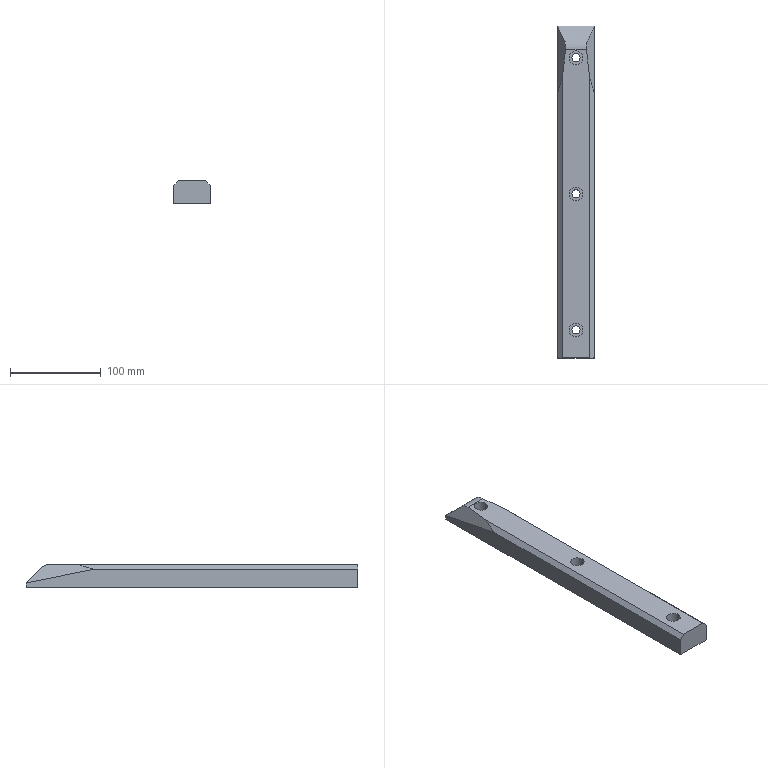Part | SolidWorks | features Chamfer 5, ICE 5, Fillet 3, HoleWzd 2, Extrusion 1, MirrorPattern 1 | 1 solid | 27 faces | box 40 x 366 x 25 mm | volume 336902 mm3 | plane 14 | cylinder 13 | commonest cylinder face diameters 9 x6 15 x6 30 x1
STEP:
#1=CARTESIAN_POINT('',(-4.5,-152.,0.));
#2=VERTEX_POINT('',#1);
#3=CARTESIAN_POINT('',(4.5,-152.,0.));
#4=VERTEX_POINT('',#3);
#5=CARTESIAN_POINT('',(0.,-152.,0.));
#6=DIRECTION('',(0.,0.,1.));
#7=DIRECTION('',(1.,0.,0.));
#8=AXIS2_PLACEMENT_3D('',#5,#6,#7);
#9=CIRCLE('',#8,4.5);
#10=EDGE_CURVE('',#2,#4,#9,.T.);
#11=ORIENTED_EDGE('',*,*,#10,.F.);
#12=CARTESIAN_POINT('',(-4.5,-152.,13.));
#13=VERTEX_POINT('',#12);
#14=CARTESIAN_POINT('',(-4.5,-152.,23.));
#15=DIRECTION('',(0.,0.,1.));
#16=VECTOR('',#15,1000.);
#17=LINE('',#14,#16);
#18=EDGE_CURVE('',#2,#13,#17,.T.);
#19=ORIENTED_EDGE('',*,*,#18,.T.);
#20=CARTESIAN_POINT('',(4.5,-152.,13.));
#21=VERTEX_POINT('',#20);
#22=CARTESIAN_POINT('',(0.,-152.,13.));
#23=DIRECTION('',(0.,0.,1.));
#24=DIRECTION('',(1.,0.,0.));
#25=AXIS2_PLACEMENT_3D('',#22,#23,#24);
#26=CIRCLE('',#25,4.5);
#27=EDGE_CURVE('',#13,#21,#26,.T.);
#28=ORIENTED_EDGE('',*,*,#27,.T.);
#29=CARTESIAN_POINT('',(4.5,-152.,23.));
#30=DIRECTION('',(0.,0.,1.));
#31=VECTOR('',#30,1000.);
#32=LINE('',#29,#31);
#33=EDGE_CURVE('',#4,#21,#32,.T.);
#34=ORIENTED_EDGE('',*,*,#33,.F.);
#35=EDGE_LOOP('',(#11,#19,#28,#34));
#36=FACE_OUTER_BOUND('',#35,.T.);
#37=CARTESIAN_POINT('',(0.,-152.,23.));
#38=DIRECTION('',(0.,0.,1.));
#39=DIRECTION('',(1.,0.,0.));
#40=AXIS2_PLACEMENT_3D('',#37,#38,#39);
#41=CYLINDRICAL_SURFACE('',#40,4.5);
#42=ADVANCED_FACE('',(#36),#41,.F.);
#43=CARTESIAN_POINT('',(-4.5,-2.,0.));
#44=VERTEX_POINT('',#43);
#45=CARTESIAN_POINT('',(4.5,-2.,0.));
#46=VERTEX_POINT('',#45);
#47=CARTESIAN_POINT('',(0.,-2.,0.));
#48=DIRECTION('',(0.,0.,1.));
#49=DIRECTION('',(1.,0.,0.));
#50=AXIS2_PLACEMENT_3D('',#47,#48,#49);
#51=CIRCLE('',#50,4.5);
#52=EDGE_CURVE('',#44,#46,#51,.T.);
#53=ORIENTED_EDGE('',*,*,#52,.F.);
#54=CARTESIAN_POINT('',(-4.5,-2.,13.));
#55=VERTEX_POINT('',#54);
#56=CARTESIAN_POINT('',(-4.5,-2.,23.));
#57=DIRECTION('',(0.,0.,1.));
#58=VECTOR('',#57,1000.);
#59=LINE('',#56,#58);
#60=EDGE_CURVE('',#44,#55,#59,.T.);
#61=ORIENTED_EDGE('',*,*,#60,.T.);
#62=CARTESIAN_POINT('',(4.5,-2.,13.));
#63=VERTEX_POINT('',#62);
#64=CARTESIAN_POINT('',(0.,-2.,13.));
#65=DIRECTION('',(0.,0.,1.));
#66=DIRECTION('',(1.,0.,0.));
#67=AXIS2_PLACEMENT_3D('',#64,#65,#66);
#68=CIRCLE('',#67,4.5);
#69=EDGE_CURVE('',#55,#63,#68,.T.);
#70=ORIENTED_EDGE('',*,*,#69,.T.);
#71=CARTESIAN_POINT('',(4.5,-2.,23.));
#72=DIRECTION('',(0.,0.,1.));
#73=VECTOR('',#72,1000.);
#74=LINE('',#71,#73);
#75=EDGE_CURVE('',#46,#63,#74,.T.);
#76=ORIENTED_EDGE('',*,*,#75,.F.);
#77=EDGE_LOOP('',(#53,#61,#70,#76));
#78=FACE_OUTER_BOUND('',#77,.T.);
#79=CARTESIAN_POINT('',(0.,-2.,23.));
#80=DIRECTION('',(0.,0.,1.));
#81=DIRECTION('',(1.,0.,0.));
#82=AXIS2_PLACEMENT_3D('',#79,#80,#81);
#83=CYLINDRICAL_SURFACE('',#82,4.5);
#84=ADVANCED_FACE('',(#78),#83,.F.);
#85=CARTESIAN_POINT('',(-4.5,148.,0.));
#86=VERTEX_POINT('',#85);
#87=CARTESIAN_POINT('',(4.5,148.,0.));
#88=VERTEX_POINT('',#87);
#89=CARTESIAN_POINT('',(0.,148.,0.));
#90=DIRECTION('',(0.,0.,1.));
#91=DIRECTION('',(1.,0.,0.));
#92=AXIS2_PLACEMENT_3D('',#89,#90,#91);
#93=CIRCLE('',#92,4.5);
#94=EDGE_CURVE('',#86,#88,#93,.T.);
#95=ORIENTED_EDGE('',*,*,#94,.F.);
#96=CARTESIAN_POINT('',(-4.5,148.,13.));
#97=VERTEX_POINT('',#96);
#98=CARTESIAN_POINT('',(-4.5,148.,23.));
#99=DIRECTION('',(0.,0.,1.));
#100=VECTOR('',#99,1000.);
#101=LINE('',#98,#100);
#102=EDGE_CURVE('',#86,#97,#101,.T.);
#103=ORIENTED_EDGE('',*,*,#102,.T.);
#104=CARTESIAN_POINT('',(4.5,148.,13.));
#105=VERTEX_POINT('',#104);
#106=CARTESIAN_POINT('',(0.,148.,13.));
#107=DIRECTION('',(0.,0.,1.));
#108=DIRECTION('',(1.,0.,0.));
#109=AXIS2_PLACEMENT_3D('',#106,#107,#108);
#110=CIRCLE('',#109,4.5);
#111=EDGE_CURVE('',#97,#105,#110,.T.);
#112=ORIENTED_EDGE('',*,*,#111,.T.);
#113=CARTESIAN_POINT('',(4.5,148.,23.));
#114=DIRECTION('',(0.,0.,1.));
#115=VECTOR('',#114,1000.);
#116=LINE('',#113,#115);
#117=EDGE_CURVE('',#88,#105,#116,.T.);
#118=ORIENTED_EDGE('',*,*,#117,.F.);
#119=EDGE_LOOP('',(#95,#103,#112,#118));
#120=FACE_OUTER_BOUND('',#119,.T.);
#121=CARTESIAN_POINT('',(0.,148.,23.));
#122=DIRECTION('',(0.,0.,1.));
#123=DIRECTION('',(1.,0.,0.));
#124=AXIS2_PLACEMENT_3D('',#121,#122,#123);
#125=CYLINDRICAL_SURFACE('',#124,4.5);
#126=ADVANCED_FACE('',(#120),#125,.F.);
#127=CARTESIAN_POINT('',(-7.5,-152.,13.));
#128=VERTEX_POINT('',#127);
#129=CARTESIAN_POINT('',(7.5,-152.,13.));
#130=VERTEX_POINT('',#129);
#131=CARTESIAN_POINT('',(0.,-152.,13.));
#132=DIRECTION('',(0.,0.,1.));
#133=DIRECTION('',(1.,0.,0.));
#134=AXIS2_PLACEMENT_3D('',#131,#132,#133);
#135=CIRCLE('',#134,7.5);
#136=EDGE_CURVE('',#128,#130,#135,.T.);
#137=ORIENTED_EDGE('',*,*,#136,.F.);
#138=CARTESIAN_POINT('',(-7.5,-152.,25.));
#139=VERTEX_POINT('',#138);
#140=CARTESIAN_POINT('',(-7.5,-152.,23.));
#141=DIRECTION('',(0.,0.,1.));
#142=VECTOR('',#141,1000.);
#143=LINE('',#140,#142);
#144=EDGE_CURVE('',#128,#139,#143,.T.);
#145=ORIENTED_EDGE('',*,*,#144,.T.);
#146=CARTESIAN_POINT('',(7.5,-152.,25.));
#147=VERTEX_POINT('',#146);
#148=CARTESIAN_POINT('',(0.,-152.,25.));
#149=DIRECTION('',(0.,0.,1.));
#150=DIRECTION('',(1.,0.,0.));
#151=AXIS2_PLACEMENT_3D('',#148,#149,#150);
#152=CIRCLE('',#151,7.5);
#153=EDGE_CURVE('',#139,#147,#152,.T.);
#154=ORIENTED_EDGE('',*,*,#153,.T.);
#155=CARTESIAN_POINT('',(7.5,-152.,23.));
#156=DIRECTION('',(0.,0.,1.));
#157=VECTOR('',#156,1000.);
#158=LINE('',#155,#157);
#159=EDGE_CURVE('',#130,#147,#158,.T.);
#160=ORIENTED_EDGE('',*,*,#159,.F.);
#161=EDGE_LOOP('',(#137,#145,#154,#160));
#162=FACE_OUTER_BOUND('',#161,.T.);
#163=CARTESIAN_POINT('',(0.,-152.,23.));
#164=DIRECTION('',(0.,0.,1.));
#165=DIRECTION('',(1.,0.,0.));
#166=AXIS2_PLACEMENT_3D('',#163,#164,#165);
#167=CYLINDRICAL_SURFACE('',#166,7.5);
#168=ADVANCED_FACE('',(#162),#167,.F.);
#169=CARTESIAN_POINT('',(-7.5,-2.,13.));
#170=VERTEX_POINT('',#169);
#171=CARTESIAN_POINT('',(7.5,-2.,13.));
#172=VERTEX_POINT('',#171);
#173=CARTESIAN_POINT('',(0.,-2.,13.));
#174=DIRECTION('',(0.,0.,1.));
#175=DIRECTION('',(1.,0.,0.));
#176=AXIS2_PLACEMENT_3D('',#173,#174,#175);
#177=CIRCLE('',#176,7.5);
#178=EDGE_CURVE('',#170,#172,#177,.T.);
#179=ORIENTED_EDGE('',*,*,#178,.F.);
#180=CARTESIAN_POINT('',(-7.5,-2.,25.));
#181=VERTEX_POINT('',#180);
#182=CARTESIAN_POINT('',(-7.5,-2.,23.));
#183=DIRECTION('',(0.,0.,1.));
#184=VECTOR('',#183,1000.);
#185=LINE('',#182,#184);
#186=EDGE_CURVE('',#170,#181,#185,.T.);
#187=ORIENTED_EDGE('',*,*,#186,.T.);
#188=CARTESIAN_POINT('',(7.5,-2.,25.));
#189=VERTEX_POINT('',#188);
#190=CARTESIAN_POINT('',(0.,-2.,25.));
#191=DIRECTION('',(0.,0.,1.));
#192=DIRECTION('',(1.,0.,0.));
#193=AXIS2_PLACEMENT_3D('',#190,#191,#192);
#194=CIRCLE('',#193,7.5);
#195=EDGE_CURVE('',#181,#189,#194,.T.);
#196=ORIENTED_EDGE('',*,*,#195,.T.);
#197=CARTESIAN_POINT('',(7.5,-2.,23.));
#198=DIRECTION('',(0.,0.,1.));
#199=VECTOR('',#198,1000.);
#200=LINE('',#197,#199);
#201=EDGE_CURVE('',#172,#189,#200,.T.);
#202=ORIENTED_EDGE('',*,*,#201,.F.);
#203=EDGE_LOOP('',(#179,#187,#196,#202));
#204=FACE_OUTER_BOUND('',#203,.T.);
#205=CARTESIAN_POINT('',(0.,-2.,23.));
#206=DIRECTION('',(0.,0.,1.));
#207=DIRECTION('',(1.,0.,0.));
#208=AXIS2_PLACEMENT_3D('',#205,#206,#207);
#209=CYLINDRICAL_SURFACE('',#208,7.5);
#210=ADVANCED_FACE('',(#204),#209,.F.);
#211=CARTESIAN_POINT('',(-7.5,148.,13.));
#212=VERTEX_POINT('',#211);
#213=CARTESIAN_POINT('',(7.5,148.,13.));
#214=VERTEX_POINT('',#213);
#215=CARTESIAN_POINT('',(0.,148.,13.));
#216=DIRECTION('',(0.,0.,1.));
#217=DIRECTION('',(1.,0.,0.));
#218=AXIS2_PLACEMENT_3D('',#215,#216,#217);
#219=CIRCLE('',#218,7.5);
#220=EDGE_CURVE('',#212,#214,#219,.T.);
#221=ORIENTED_EDGE('',*,*,#220,.F.);
#222=CARTESIAN_POINT('',(-7.5,148.,25.));
#223=VERTEX_POINT('',#222);
#224=CARTESIAN_POINT('',(-7.5,148.,23.));
#225=DIRECTION('',(0.,0.,1.));
#226=VECTOR('',#225,1000.);
#227=LINE('',#224,#226);
#228=EDGE_CURVE('',#212,#223,#227,.T.);
#229=ORIENTED_EDGE('',*,*,#228,.T.);
#230=CARTESIAN_POINT('',(7.5,148.,25.));
#231=VERTEX_POINT('',#230);
#232=CARTESIAN_POINT('',(0.,148.,25.));
#233=DIRECTION('',(0.,0.,1.));
#234=DIRECTION('',(1.,0.,0.));
#235=AXIS2_PLACEMENT_3D('',#232,#233,#234);
#236=CIRCLE('',#235,7.5);
#237=EDGE_CURVE('',#223,#231,#236,.T.);
#238=ORIENTED_EDGE('',*,*,#237,.T.);
#239=CARTESIAN_POINT('',(7.5,148.,23.));
#240=DIRECTION('',(0.,0.,1.));
#241=VECTOR('',#240,1000.);
#242=LINE('',#239,#241);
#243=EDGE_CURVE('',#214,#231,#242,.T.);
#244=ORIENTED_EDGE('',*,*,#243,.F.);
#245=EDGE_LOOP('',(#221,#229,#238,#244));
#246=FACE_OUTER_BOUND('',#245,.T.);
#247=CARTESIAN_POINT('',(0.,148.,23.));
#248=DIRECTION('',(0.,0.,1.));
#249=DIRECTION('',(1.,0.,0.));
#250=AXIS2_PLACEMENT_3D('',#247,#248,#249);
#251=CYLINDRICAL_SURFACE('',#250,7.5);
#252=ADVANCED_FACE('',(#246),#251,.F.);
#253=CARTESIAN_POINT('',(-20.,183.,5.));
#254=VERTEX_POINT('',#253);
#255=CARTESIAN_POINT('',(-20.,183.,0.));
#256=VERTEX_POINT('',#255);
#257=CARTESIAN_POINT('',(-20.,183.,25.));
#258=DIRECTION('',(0.,0.,-1.));
#259=VECTOR('',#258,1000.);
#260=LINE('',#257,#259);
#261=EDGE_CURVE('',#254,#256,#260,.T.);
#262=ORIENTED_EDGE('',*,*,#261,.F.);
#263=CARTESIAN_POINT('',(20.,183.,5.));
#264=VERTEX_POINT('',#263);
#265=CARTESIAN_POINT('',(20.,183.,5.));
#266=DIRECTION('',(-1.,0.,0.));
#267=VECTOR('',#266,1000.);
#268=LINE('',#265,#267);
#269=EDGE_CURVE('',#264,#254,#268,.T.);
#270=ORIENTED_EDGE('',*,*,#269,.F.);
#271=CARTESIAN_POINT('',(20.,183.,0.));
#272=VERTEX_POINT('',#271);
#273=CARTESIAN_POINT('',(20.,183.,25.));
#274=DIRECTION('',(0.,0.,-1.));
#275=VECTOR('',#274,1000.);
#276=LINE('',#273,#275);
#277=EDGE_CURVE('',#264,#272,#276,.T.);
#278=ORIENTED_EDGE('',*,*,#277,.T.);
#279=CARTESIAN_POINT('',(-20.,183.,0.));
#280=DIRECTION('',(-1.,0.,0.));
#281=VECTOR('',#280,1000.);
#282=LINE('',#279,#281);
#283=EDGE_CURVE('',#272,#256,#282,.T.);
#284=ORIENTED_EDGE('',*,*,#283,.T.);
#285=EDGE_LOOP('',(#262,#270,#278,#284));
#286=FACE_OUTER_BOUND('',#285,.T.);
#287=CARTESIAN_POINT('',(-20.,183.,25.));
#288=DIRECTION('',(0.,-1.,0.));
#289=DIRECTION('',(0.,0.,-1.));
#290=AXIS2_PLACEMENT_3D('',#287,#288,#289);
#291=PLANE('',#290);
#292=ADVANCED_FACE('',(#286),#291,.F.);
#293=CARTESIAN_POINT('',(15.,126.301,25.));
#294=VERTEX_POINT('',#293);
#295=CARTESIAN_POINT('',(11.48,156.787,25.));
#296=VERTEX_POINT('',#295);
#297=CARTESIAN_POINT('',(20.,83.,25.));
#298=DIRECTION('',(-0.1147,0.9934,0.));
#299=VECTOR('',#298,1000.);
#300=LINE('',#297,#299);
#301=EDGE_CURVE('',#294,#296,#300,.T.);
#302=ORIENTED_EDGE('',*,*,#301,.T.);
#303=CARTESIAN_POINT('',(-11.48,156.787,25.));
#304=VERTEX_POINT('',#303);
#305=CARTESIAN_POINT('',(-10.762,156.787,25.));
#306=DIRECTION('',(-1.,0.,0.));
#307=VECTOR('',#306,1000.);
#308=LINE('',#305,#307);
#309=EDGE_CURVE('',#296,#304,#308,.T.);
#310=ORIENTED_EDGE('',*,*,#309,.T.);
#311=CARTESIAN_POINT('',(-15.,126.301,25.));
#312=VERTEX_POINT('',#311);
#313=CARTESIAN_POINT('',(-20.,83.,25.));
#314=DIRECTION('',(0.1147,0.9934,0.));
#315=VECTOR('',#314,1000.);
#316=LINE('',#313,#315);
#317=EDGE_CURVE('',#312,#304,#316,.T.);
#318=ORIENTED_EDGE('',*,*,#317,.F.);
#319=CARTESIAN_POINT('',(-15.,-183.,25.));
#320=VERTEX_POINT('',#319);
#321=CARTESIAN_POINT('',(-15.,-183.,25.));
#322=DIRECTION('',(0.,-1.,0.));
#323=VECTOR('',#322,1000.);
#324=LINE('',#321,#323);
#325=EDGE_CURVE('',#312,#320,#324,.T.);
#326=ORIENTED_EDGE('',*,*,#325,.T.);
#327=CARTESIAN_POINT('',(15.,-183.,25.));
#328=VERTEX_POINT('',#327);
#329=CARTESIAN_POINT('',(-20.,-183.,25.));
#330=DIRECTION('',(1.,0.,0.));
#331=VECTOR('',#330,1000.);
#332=LINE('',#329,#331);
#333=EDGE_CURVE('',#320,#328,#332,.T.);
#334=ORIENTED_EDGE('',*,*,#333,.T.);
#335=CARTESIAN_POINT('',(15.,83.,25.));
#336=DIRECTION('',(0.,1.,0.));
#337=VECTOR('',#336,1000.);
#338=LINE('',#335,#337);
#339=EDGE_CURVE('',#328,#294,#338,.T.);
#340=ORIENTED_EDGE('',*,*,#339,.T.);
#341=EDGE_LOOP('',(#302,#310,#318,#326,#334,#340));
#342=FACE_OUTER_BOUND('',#341,.T.);
#343=CARTESIAN_POINT('',(0.,-152.,25.));
#344=DIRECTION('',(0.,0.,1.));
#345=DIRECTION('',(1.,0.,0.));
#346=AXIS2_PLACEMENT_3D('',#343,#344,#345);
#347=CIRCLE('',#346,7.5);
#348=EDGE_CURVE('',#147,#139,#347,.T.);
#349=ORIENTED_EDGE('',*,*,#348,.F.);
#350=ORIENTED_EDGE('',*,*,#153,.F.);
#351=EDGE_LOOP('',(#349,#350));
#352=FACE_BOUND('',#351,.T.);
#353=CARTESIAN_POINT('',(0.,-2.,25.));
#354=DIRECTION('',(0.,0.,1.));
#355=DIRECTION('',(1.,0.,0.));
#356=AXIS2_PLACEMENT_3D('',#353,#354,#355);
#357=CIRCLE('',#356,7.5);
#358=EDGE_CURVE('',#189,#181,#357,.T.);
#359=ORIENTED_EDGE('',*,*,#358,.F.);
#360=ORIENTED_EDGE('',*,*,#195,.F.);
#361=EDGE_LOOP('',(#359,#360));
#362=FACE_BOUND('',#361,.T.);
#363=CARTESIAN_POINT('',(0.,148.,25.));
#364=DIRECTION('',(0.,0.,1.));
#365=DIRECTION('',(1.,0.,0.));
#366=AXIS2_PLACEMENT_3D('',#363,#364,#365);
#367=CIRCLE('',#366,7.5);
#368=EDGE_CURVE('',#231,#223,#367,.T.);
#369=ORIENTED_EDGE('',*,*,#368,.F.);
#370=ORIENTED_EDGE('',*,*,#237,.F.);
#371=EDGE_LOOP('',(#369,#370));
#372=FACE_BOUND('',#371,.T.);
#373=CARTESIAN_POINT('',(0.,0.,25.));
#374=DIRECTION('',(0.,0.,1.));
#375=DIRECTION('',(1.,0.,0.));
#376=AXIS2_PLACEMENT_3D('',#373,#374,#375);
#377=PLANE('',#376);
#378=ADVANCED_FACE('',(#342,#352,#362,#372),#377,.T.);
#379=CARTESIAN_POINT('',(20.,108.,20.));
#380=VERTEX_POINT('',#379);
#381=CARTESIAN_POINT('',(20.,183.,5.));
#382=DIRECTION('',(0.,-0.9806,0.1961));
#383=VECTOR('',#382,1000.);
#384=LINE('',#381,#383);
#385=EDGE_CURVE('',#264,#380,#384,.T.);
#386=ORIENTED_EDGE('',*,*,#385,.T.);
#387=CARTESIAN_POINT('',(20.,-183.,20.));
#388=VERTEX_POINT('',#387);
#389=CARTESIAN_POINT('',(20.,-183.,20.));
#390=DIRECTION('',(0.,-1.,0.));
#391=VECTOR('',#390,1000.);
#392=LINE('',#389,#391);
#393=EDGE_CURVE('',#380,#388,#392,.T.);
#394=ORIENTED_EDGE('',*,*,#393,.T.);
#395=CARTESIAN_POINT('',(20.,-183.,0.));
#396=VERTEX_POINT('',#395);
#397=CARTESIAN_POINT('',(20.,-183.,25.));
#398=DIRECTION('',(0.,0.,-1.));
#399=VECTOR('',#398,1000.);
#400=LINE('',#397,#399);
#401=EDGE_CURVE('',#388,#396,#400,.T.);
#402=ORIENTED_EDGE('',*,*,#401,.T.);
#403=CARTESIAN_POINT('',(20.,183.,0.));
#404=DIRECTION('',(0.,1.,0.));
#405=VECTOR('',#404,1000.);
#406=LINE('',#403,#405);
#407=EDGE_CURVE('',#396,#272,#406,.T.);
#408=ORIENTED_EDGE('',*,*,#407,.T.);
#409=ORIENTED_EDGE('',*,*,#277,.F.);
#410=EDGE_LOOP('',(#386,#394,#402,#408,#409));
#411=FACE_OUTER_BOUND('',#410,.T.);
#412=CARTESIAN_POINT('',(20.,183.,25.));
#413=DIRECTION('',(-1.,0.,0.));
#414=DIRECTION('',(0.,-1.,0.));
#415=AXIS2_PLACEMENT_3D('',#412,#413,#414);
#416=PLANE('',#415);
#417=ADVANCED_FACE('',(#411),#416,.F.);
#418=CARTESIAN_POINT('',(-20.,-183.,20.));
#419=VERTEX_POINT('',#418);
#420=CARTESIAN_POINT('',(-20.,-183.,0.));
#421=VERTEX_POINT('',#420);
#422=CARTESIAN_POINT('',(-20.,-183.,25.));
#423=DIRECTION('',(0.,0.,-1.));
#424=VECTOR('',#423,1000.);
#425=LINE('',#422,#424);
#426=EDGE_CURVE('',#419,#421,#425,.T.);
#427=ORIENTED_EDGE('',*,*,#426,.F.);
#428=CARTESIAN_POINT('',(-20.,108.,20.));
#429=VERTEX_POINT('',#428);
#430=CARTESIAN_POINT('',(-20.,83.,20.));
#431=DIRECTION('',(0.,1.,0.));
#432=VECTOR('',#431,1000.);
#433=LINE('',#430,#432);
#434=EDGE_CURVE('',#419,#429,#433,.T.);
#435=ORIENTED_EDGE('',*,*,#434,.T.);
#436=CARTESIAN_POINT('',(-20.,183.,5.));
#437=DIRECTION('',(0.,-0.9806,0.1961));
#438=VECTOR('',#437,1000.);
#439=LINE('',#436,#438);
#440=EDGE_CURVE('',#254,#429,#439,.T.);
#441=ORIENTED_EDGE('',*,*,#440,.F.);
#442=ORIENTED_EDGE('',*,*,#261,.T.);
#443=CARTESIAN_POINT('',(-20.,183.,0.));
#444=DIRECTION('',(0.,-1.,0.));
#445=VECTOR('',#444,1000.);
#446=LINE('',#443,#445);
#447=EDGE_CURVE('',#256,#421,#446,.T.);
#448=ORIENTED_EDGE('',*,*,#447,.T.);
#449=EDGE_LOOP('',(#427,#435,#441,#442,#448));
#450=FACE_OUTER_BOUND('',#449,.T.);
#451=CARTESIAN_POINT('',(-20.,183.,25.));
#452=DIRECTION('',(1.,0.,0.));
#453=DIRECTION('',(0.,1.,0.));
#454=AXIS2_PLACEMENT_3D('',#451,#452,#453);
#455=PLANE('',#454);
#456=ADVANCED_FACE('',(#450),#455,.F.);
#457=ORIENTED_EDGE('',*,*,#401,.F.);
#458=CARTESIAN_POINT('',(15.,-183.,25.));
#459=DIRECTION('',(-0.7071,0.,0.7071));
#460=VECTOR('',#459,1000.);
#461=LINE('',#458,#460);
#462=EDGE_CURVE('',#388,#328,#461,.T.);
#463=ORIENTED_EDGE('',*,*,#462,.T.);
#464=ORIENTED_EDGE('',*,*,#333,.F.);
#465=CARTESIAN_POINT('',(-15.,-183.,25.));
#466=DIRECTION('',(-0.7071,0.,-0.7071));
#467=VECTOR('',#466,1000.);
#468=LINE('',#465,#467);
#469=EDGE_CURVE('',#320,#419,#468,.T.);
#470=ORIENTED_EDGE('',*,*,#469,.T.);
#471=ORIENTED_EDGE('',*,*,#426,.T.);
#472=CARTESIAN_POINT('',(-20.,-183.,0.));
#473=DIRECTION('',(1.,0.,0.));
#474=VECTOR('',#473,1000.);
#475=LINE('',#472,#474);
#476=EDGE_CURVE('',#421,#396,#475,.T.);
#477=ORIENTED_EDGE('',*,*,#476,.T.);
#478=EDGE_LOOP('',(#457,#463,#464,#470,#471,#477));
#479=FACE_OUTER_BOUND('',#478,.T.);
#480=CARTESIAN_POINT('',(-20.,-183.,25.));
#481=DIRECTION('',(0.,1.,0.));
#482=DIRECTION('',(0.,0.,1.));
#483=AXIS2_PLACEMENT_3D('',#480,#481,#482);
#484=PLANE('',#483);
#485=ADVANCED_FACE('',(#479),#484,.F.);
#486=CARTESIAN_POINT('',(0.,-152.,0.));
#487=DIRECTION('',(0.,0.,1.));
#488=DIRECTION('',(1.,0.,0.));
#489=AXIS2_PLACEMENT_3D('',#486,#487,#488);
#490=CIRCLE('',#489,4.5);
#491=EDGE_CURVE('',#4,#2,#490,.T.);
#492=ORIENTED_EDGE('',*,*,#491,.T.);
#493=ORIENTED_EDGE('',*,*,#10,.T.);
#494=EDGE_LOOP('',(#492,#493));
#495=FACE_BOUND('',#494,.T.);
#496=CARTESIAN_POINT('',(0.,-2.,0.));
#497=DIRECTION('',(0.,0.,1.));
#498=DIRECTION('',(1.,0.,0.));
#499=AXIS2_PLACEMENT_3D('',#496,#497,#498);
#500=CIRCLE('',#499,4.5);
#501=EDGE_CURVE('',#46,#44,#500,.T.);
#502=ORIENTED_EDGE('',*,*,#501,.T.);
#503=ORIENTED_EDGE('',*,*,#52,.T.);
#504=EDGE_LOOP('',(#502,#503));
#505=FACE_BOUND('',#504,.T.);
#506=CARTESIAN_POINT('',(0.,148.,0.));
#507=DIRECTION('',(0.,0.,1.));
#508=DIRECTION('',(1.,0.,0.));
#509=AXIS2_PLACEMENT_3D('',#506,#507,#508);
#510=CIRCLE('',#509,4.5);
#511=EDGE_CURVE('',#88,#86,#510,.T.);
#512=ORIENTED_EDGE('',*,*,#511,.T.);
#513=ORIENTED_EDGE('',*,*,#94,.T.);
#514=EDGE_LOOP('',(#512,#513));
#515=FACE_BOUND('',#514,.T.);
#516=ORIENTED_EDGE('',*,*,#407,.F.);
#517=ORIENTED_EDGE('',*,*,#476,.F.);
#518=ORIENTED_EDGE('',*,*,#447,.F.);
#519=ORIENTED_EDGE('',*,*,#283,.F.);
#520=EDGE_LOOP('',(#516,#517,#518,#519));
#521=FACE_OUTER_BOUND('',#520,.T.);
#522=CARTESIAN_POINT('',(0.,0.,0.));
#523=DIRECTION('',(0.,0.,1.));
#524=DIRECTION('',(1.,0.,0.));
#525=AXIS2_PLACEMENT_3D('',#522,#523,#524);
#526=PLANE('',#525);
#527=ADVANCED_FACE('',(#495,#505,#515,#521),#526,.F.);
#528=ORIENTED_EDGE('',*,*,#228,.F.);
#529=CARTESIAN_POINT('',(0.,148.,13.));
#530=DIRECTION('',(0.,0.,1.));
#531=DIRECTION('',(1.,0.,0.));
#532=AXIS2_PLACEMENT_3D('',#529,#530,#531);
#533=CIRCLE('',#532,7.5);
#534=EDGE_CURVE('',#214,#212,#533,.T.);
#535=ORIENTED_EDGE('',*,*,#534,.F.);
#536=ORIENTED_EDGE('',*,*,#243,.T.);
#537=ORIENTED_EDGE('',*,*,#368,.T.);
#538=EDGE_LOOP('',(#528,#535,#536,#537));
#539=FACE_OUTER_BOUND('',#538,.T.);
#540=CARTESIAN_POINT('',(0.,148.,23.));
#541=DIRECTION('',(0.,0.,1.));
#542=DIRECTION('',(1.,0.,0.));
#543=AXIS2_PLACEMENT_3D('',#540,#541,#542);
#544=CYLINDRICAL_SURFACE('',#543,7.5);
#545=ADVANCED_FACE('',(#539),#544,.F.);
#546=ORIENTED_EDGE('',*,*,#186,.F.);
#547=CARTESIAN_POINT('',(0.,-2.,13.));
#548=DIRECTION('',(0.,0.,1.));
#549=DIRECTION('',(1.,0.,0.));
#550=AXIS2_PLACEMENT_3D('',#547,#548,#549);
#551=CIRCLE('',#550,7.5);
#552=EDGE_CURVE('',#172,#170,#551,.T.);
#553=ORIENTED_EDGE('',*,*,#552,.F.);
#554=ORIENTED_EDGE('',*,*,#201,.T.);
#555=ORIENTED_EDGE('',*,*,#358,.T.);
#556=EDGE_LOOP('',(#546,#553,#554,#555));
#557=FACE_OUTER_BOUND('',#556,.T.);
#558=CARTESIAN_POINT('',(0.,-2.,23.));
#559=DIRECTION('',(0.,0.,1.));
#560=DIRECTION('',(1.,0.,0.));
#561=AXIS2_PLACEMENT_3D('',#558,#559,#560);
#562=CYLINDRICAL_SURFACE('',#561,7.5);
#563=ADVANCED_FACE('',(#557),#562,.F.);
#564=ORIENTED_EDGE('',*,*,#144,.F.);
#565=CARTESIAN_POINT('',(0.,-152.,13.));
#566=DIRECTION('',(0.,0.,1.));
#567=DIRECTION('',(1.,0.,0.));
#568=AXIS2_PLACEMENT_3D('',#565,#566,#567);
#569=CIRCLE('',#568,7.5);
#570=EDGE_CURVE('',#130,#128,#569,.T.);
#571=ORIENTED_EDGE('',*,*,#570,.F.);
#572=ORIENTED_EDGE('',*,*,#159,.T.);
#573=ORIENTED_EDGE('',*,*,#348,.T.);
#574=EDGE_LOOP('',(#564,#571,#572,#573));
#575=FACE_OUTER_BOUND('',#574,.T.);
#576=CARTESIAN_POINT('',(0.,-152.,23.));
#577=DIRECTION('',(0.,0.,1.));
#578=DIRECTION('',(1.,0.,0.));
#579=AXIS2_PLACEMENT_3D('',#576,#577,#578);
#580=CYLINDRICAL_SURFACE('',#579,7.5);
#581=ADVANCED_FACE('',(#575),#580,.F.);
#582=ORIENTED_EDGE('',*,*,#102,.F.);
#583=ORIENTED_EDGE('',*,*,#511,.F.);
#584=ORIENTED_EDGE('',*,*,#117,.T.);
#585=CARTESIAN_POINT('',(0.,148.,13.));
#586=DIRECTION('',(0.,0.,1.));
#587=DIRECTION('',(1.,0.,0.));
#588=AXIS2_PLACEMENT_3D('',#585,#586,#587);
#589=CIRCLE('',#588,4.5);
#590=EDGE_CURVE('',#105,#97,#589,.T.);
#591=ORIENTED_EDGE('',*,*,#590,.T.);
#592=EDGE_LOOP('',(#582,#583,#584,#591));
#593=FACE_OUTER_BOUND('',#592,.T.);
#594=CARTESIAN_POINT('',(0.,148.,23.));
#595=DIRECTION('',(0.,0.,1.));
#596=DIRECTION('',(1.,0.,0.));
#597=AXIS2_PLACEMENT_3D('',#594,#595,#596);
#598=CYLINDRICAL_SURFACE('',#597,4.5);
#599=ADVANCED_FACE('',(#593),#598,.F.);
#600=ORIENTED_EDGE('',*,*,#590,.F.);
#601=ORIENTED_EDGE('',*,*,#111,.F.);
#602=EDGE_LOOP('',(#600,#601));
#603=FACE_BOUND('',#602,.T.);
#604=ORIENTED_EDGE('',*,*,#534,.T.);
#605=ORIENTED_EDGE('',*,*,#220,.T.);
#606=EDGE_LOOP('',(#604,#605));
#607=FACE_OUTER_BOUND('',#606,.T.);
#608=CARTESIAN_POINT('',(4.5,148.,13.));
#609=DIRECTION('',(0.,0.,-1.));
#610=DIRECTION('',(-1.,0.,0.));
#611=AXIS2_PLACEMENT_3D('',#608,#609,#610);
#612=PLANE('',#611);
#613=ADVANCED_FACE('',(#603,#607),#612,.F.);
#614=ORIENTED_EDGE('',*,*,#60,.F.);
#615=ORIENTED_EDGE('',*,*,#501,.F.);
#616=ORIENTED_EDGE('',*,*,#75,.T.);
#617=CARTESIAN_POINT('',(0.,-2.,13.));
#618=DIRECTION('',(0.,0.,1.));
#619=DIRECTION('',(1.,0.,0.));
#620=AXIS2_PLACEMENT_3D('',#617,#618,#619);
#621=CIRCLE('',#620,4.5);
#622=EDGE_CURVE('',#63,#55,#621,.T.);
#623=ORIENTED_EDGE('',*,*,#622,.T.);
#624=EDGE_LOOP('',(#614,#615,#616,#623));
#625=FACE_OUTER_BOUND('',#624,.T.);
#626=CARTESIAN_POINT('',(0.,-2.,23.));
#627=DIRECTION('',(0.,0.,1.));
#628=DIRECTION('',(1.,0.,0.));
#629=AXIS2_PLACEMENT_3D('',#626,#627,#628);
#630=CYLINDRICAL_SURFACE('',#629,4.5);
#631=ADVANCED_FACE('',(#625),#630,.F.);
#632=ORIENTED_EDGE('',*,*,#622,.F.);
#633=ORIENTED_EDGE('',*,*,#69,.F.);
#634=EDGE_LOOP('',(#632,#633));
#635=FACE_BOUND('',#634,.T.);
#636=ORIENTED_EDGE('',*,*,#552,.T.);
#637=ORIENTED_EDGE('',*,*,#178,.T.);
#638=EDGE_LOOP('',(#636,#637));
#639=FACE_OUTER_BOUND('',#638,.T.);
#640=CARTESIAN_POINT('',(4.5,-2.,13.));
#641=DIRECTION('',(0.,0.,-1.));
#642=DIRECTION('',(-1.,0.,0.));
#643=AXIS2_PLACEMENT_3D('',#640,#641,#642);
#644=PLANE('',#643);
#645=ADVANCED_FACE('',(#635,#639),#644,.F.);
#646=ORIENTED_EDGE('',*,*,#18,.F.);
#647=ORIENTED_EDGE('',*,*,#491,.F.);
#648=ORIENTED_EDGE('',*,*,#33,.T.);
#649=CARTESIAN_POINT('',(0.,-152.,13.));
#650=DIRECTION('',(0.,0.,1.));
#651=DIRECTION('',(1.,0.,0.));
#652=AXIS2_PLACEMENT_3D('',#649,#650,#651);
#653=CIRCLE('',#652,4.5);
#654=EDGE_CURVE('',#21,#13,#653,.T.);
#655=ORIENTED_EDGE('',*,*,#654,.T.);
#656=EDGE_LOOP('',(#646,#647,#648,#655));
#657=FACE_OUTER_BOUND('',#656,.T.);
#658=CARTESIAN_POINT('',(0.,-152.,23.));
#659=DIRECTION('',(0.,0.,1.));
#660=DIRECTION('',(1.,0.,0.));
#661=AXIS2_PLACEMENT_3D('',#658,#659,#660);
#662=CYLINDRICAL_SURFACE('',#661,4.5);
#663=ADVANCED_FACE('',(#657),#662,.F.);
#664=ORIENTED_EDGE('',*,*,#654,.F.);
#665=ORIENTED_EDGE('',*,*,#27,.F.);
#666=EDGE_LOOP('',(#664,#665));
#667=FACE_BOUND('',#666,.T.);
#668=ORIENTED_EDGE('',*,*,#570,.T.);
#669=ORIENTED_EDGE('',*,*,#136,.T.);
#670=EDGE_LOOP('',(#668,#669));
#671=FACE_OUTER_BOUND('',#670,.T.);
#672=CARTESIAN_POINT('',(4.5,-152.,13.));
#673=DIRECTION('',(0.,0.,-1.));
#674=DIRECTION('',(-1.,0.,0.));
#675=AXIS2_PLACEMENT_3D('',#672,#673,#674);
#676=PLANE('',#675);
#677=ADVANCED_FACE('',(#667,#671),#676,.F.);
#678=ORIENTED_EDGE('',*,*,#317,.T.);
#679=CARTESIAN_POINT('',(-12.792,167.393,20.607));
#680=VERTEX_POINT('',#679);
#681=CARTESIAN_POINT('',(-11.48,156.787,25.));
#682=CARTESIAN_POINT('',(-11.014,160.818,25.));
#683=CARTESIAN_POINT('',(-11.475,164.543,23.457));
#684=CARTESIAN_POINT('',(-12.792,167.393,20.607));
#685=(BOUNDED_CURVE()B_SPLINE_CURVE(3,(#681,#682,#683,#684),.UNSPECIFIED.,.F.,.F.)B_SPLINE_CURVE_WITH_KNOTS((4,4),(6.086,6.871),.UNSPECIFIED.)CURVE()GEOMETRIC_REPRESENTATION_ITEM()RATIONAL_B_SPLINE_CURVE((1.,0.9493,0.9493,1.))REPRESENTATION_ITEM(''));
#686=EDGE_CURVE('',#304,#680,#685,.T.);
#687=ORIENTED_EDGE('',*,*,#686,.T.);
#688=CARTESIAN_POINT('',(19.073,98.405,89.595));
#689=DIRECTION('',(0.3105,-0.6722,0.6722));
#690=VECTOR('',#689,1000.);
#691=LINE('',#688,#690);
#692=EDGE_CURVE('',#254,#680,#691,.T.);
#693=ORIENTED_EDGE('',*,*,#692,.F.);
#694=ORIENTED_EDGE('',*,*,#440,.T.);
#695=CARTESIAN_POINT('',(-45.674,14.028,-5.674));
#696=DIRECTION('',(0.2548,0.9328,0.2548));
#697=VECTOR('',#696,1000.);
#698=LINE('',#695,#697);
#699=EDGE_CURVE('',#429,#312,#698,.T.);
#700=ORIENTED_EDGE('',*,*,#699,.T.);
#701=EDGE_LOOP('',(#678,#687,#693,#694,#700));
#702=FACE_OUTER_BOUND('',#701,.T.);
#703=CARTESIAN_POINT('',(-32.686,3.774,18.872));
#704=DIRECTION('',(-0.8617,0.0995,0.4975));
#705=DIRECTION('',(0.5,0.,0.866));
#706=AXIS2_PLACEMENT_3D('',#703,#704,#705);
#707=PLANE('',#706);
#708=ADVANCED_FACE('',(#702),#707,.T.);
#709=CARTESIAN_POINT('',(12.792,167.393,20.607));
#710=VERTEX_POINT('',#709);
#711=CARTESIAN_POINT('',(-19.073,98.405,89.595));
#712=DIRECTION('',(0.3105,0.6722,-0.6722));
#713=VECTOR('',#712,1000.);
#714=LINE('',#711,#713);
#715=EDGE_CURVE('',#710,#264,#714,.T.);
#716=ORIENTED_EDGE('',*,*,#715,.F.);
#717=CARTESIAN_POINT('',(12.792,167.393,20.607));
#718=CARTESIAN_POINT('',(11.475,164.543,23.457));
#719=CARTESIAN_POINT('',(11.014,160.818,25.));
#720=CARTESIAN_POINT('',(11.48,156.787,25.));
#721=(BOUNDED_CURVE()B_SPLINE_CURVE(3,(#717,#718,#719,#720),.UNSPECIFIED.,.F.,.F.)B_SPLINE_CURVE_WITH_KNOTS((4,4),(2.554,3.339),.UNSPECIFIED.)CURVE()GEOMETRIC_REPRESENTATION_ITEM()RATIONAL_B_SPLINE_CURVE((1.,0.9493,0.9493,1.))REPRESENTATION_ITEM(''));
#722=EDGE_CURVE('',#710,#296,#721,.T.);
#723=ORIENTED_EDGE('',*,*,#722,.T.);
#724=ORIENTED_EDGE('',*,*,#301,.F.);
#725=CARTESIAN_POINT('',(45.674,14.028,-5.674));
#726=DIRECTION('',(0.2548,-0.9328,-0.2548));
#727=VECTOR('',#726,1000.);
#728=LINE('',#725,#727);
#729=EDGE_CURVE('',#294,#380,#728,.T.);
#730=ORIENTED_EDGE('',*,*,#729,.T.);
#731=ORIENTED_EDGE('',*,*,#385,.F.);
#732=EDGE_LOOP('',(#716,#723,#724,#730,#731));
#733=FACE_OUTER_BOUND('',#732,.T.);
#734=CARTESIAN_POINT('',(32.686,3.774,18.872));
#735=DIRECTION('',(0.8617,0.0995,0.4975));
#736=DIRECTION('',(-0.5,0.,0.866));
#737=AXIS2_PLACEMENT_3D('',#734,#735,#736);
#738=PLANE('',#737);
#739=ADVANCED_FACE('',(#733),#738,.T.);
#740=ORIENTED_EDGE('',*,*,#462,.F.);
#741=ORIENTED_EDGE('',*,*,#393,.F.);
#742=ORIENTED_EDGE('',*,*,#729,.F.);
#743=ORIENTED_EDGE('',*,*,#339,.F.);
#744=EDGE_LOOP('',(#740,#741,#742,#743));
#745=FACE_OUTER_BOUND('',#744,.T.);
#746=CARTESIAN_POINT('',(15.,0.,25.));
#747=DIRECTION('',(0.7071,0.,0.7071));
#748=DIRECTION('',(0.,-1.,0.));
#749=AXIS2_PLACEMENT_3D('',#746,#747,#748);
#750=PLANE('',#749);
#751=ADVANCED_FACE('',(#745),#750,.T.);
#752=ORIENTED_EDGE('',*,*,#699,.F.);
#753=ORIENTED_EDGE('',*,*,#434,.F.);
#754=ORIENTED_EDGE('',*,*,#469,.F.);
#755=ORIENTED_EDGE('',*,*,#325,.F.);
#756=EDGE_LOOP('',(#752,#753,#754,#755));
#757=FACE_OUTER_BOUND('',#756,.T.);
#758=CARTESIAN_POINT('',(-15.,0.,25.));
#759=DIRECTION('',(-0.7071,0.,0.7071));
#760=DIRECTION('',(0.,1.,0.));
#761=AXIS2_PLACEMENT_3D('',#758,#759,#760);
#762=PLANE('',#761);
#763=ADVANCED_FACE('',(#757),#762,.T.);
#764=ORIENTED_EDGE('',*,*,#692,.T.);
#765=CARTESIAN_POINT('',(10.762,167.393,20.607));
#766=DIRECTION('',(1.,0.,0.));
#767=VECTOR('',#766,1000.);
#768=LINE('',#765,#767);
#769=EDGE_CURVE('',#680,#710,#768,.T.);
#770=ORIENTED_EDGE('',*,*,#769,.T.);
#771=ORIENTED_EDGE('',*,*,#715,.T.);
#772=ORIENTED_EDGE('',*,*,#269,.T.);
#773=EDGE_LOOP('',(#764,#770,#771,#772));
#774=FACE_OUTER_BOUND('',#773,.T.);
#775=CARTESIAN_POINT('',(20.,183.,5.));
#776=DIRECTION('',(0.,-0.7071,-0.7071));
#777=DIRECTION('',(0.,0.7071,-0.7071));
#778=AXIS2_PLACEMENT_3D('',#775,#776,#777);
#779=PLANE('',#778);
#780=ADVANCED_FACE('',(#774),#779,.F.);
#781=ORIENTED_EDGE('',*,*,#722,.F.);
#782=ORIENTED_EDGE('',*,*,#769,.F.);
#783=ORIENTED_EDGE('',*,*,#686,.F.);
#784=ORIENTED_EDGE('',*,*,#309,.F.);
#785=EDGE_LOOP('',(#781,#782,#783,#784));
#786=FACE_OUTER_BOUND('',#785,.T.);
#787=CARTESIAN_POINT('',(0.,156.787,10.));
#788=DIRECTION('',(1.,0.,0.));
#789=DIRECTION('',(0.,1.,0.));
#790=AXIS2_PLACEMENT_3D('',#787,#788,#789);
#791=CYLINDRICAL_SURFACE('',#790,15.);
#792=ADVANCED_FACE('',(#786),#791,.T.);
#793=CLOSED_SHELL('',(#42,#84,#126,#168,#210,#252,#292,#378,#417,#456,#485,#527,#545,#563,#581,#599,#613,#631,#645,#663,#677,#708,#739,#751,#763,#780,#792));
#794=MANIFOLD_SOLID_BREP('',#793);
#795=CARTESIAN_POINT('',(0.,0.,0.));
#796=DIRECTION('',(0.,0.,1.));
#797=DIRECTION('',(1.,0.,0.));
#798=AXIS2_PLACEMENT_3D('',#795,#796,#797);
#799=(LENGTH_UNIT()NAMED_UNIT(*)SI_UNIT(.MILLI.,.METRE.));
#800=UNCERTAINTY_MEASURE_WITH_UNIT(LENGTH_MEASURE(0.00001),#799,'','');
#801=(NAMED_UNIT(*)PLANE_ANGLE_UNIT()SI_UNIT($,.RADIAN.));
#802=(NAMED_UNIT(*)SI_UNIT($,.STERADIAN.)SOLID_ANGLE_UNIT());
#803=(GEOMETRIC_REPRESENTATION_CONTEXT(3)GLOBAL_UNCERTAINTY_ASSIGNED_CONTEXT((#800))GLOBAL_UNIT_ASSIGNED_CONTEXT((#799,#801,#802))REPRESENTATION_CONTEXT('',''));
#804=ADVANCED_BREP_SHAPE_REPRESENTATION('',(#794,#798),#803);